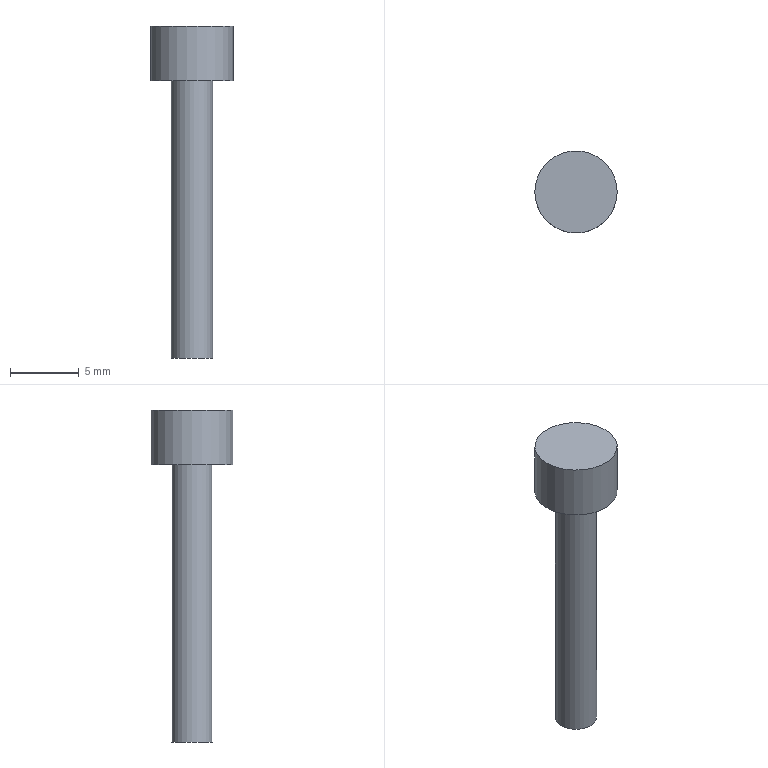Part | STEP file | 1 solid | 5 faces | box 6 x 6 x 24.2 mm | volume 255.883 mm3 | plane 3 | cylinder 2 | commonest cylinder face diameters 3 x1 6 x1
STEP:
#1=CARTESIAN_POINT('',(0.,0.,0.));
#2=DIRECTION('',(0.,0.,1.));
#3=DIRECTION('',(1.,0.,0.));
#4=AXIS2_PLACEMENT_3D('',#1,#2,#3);
#5=CARTESIAN_POINT('',(1542.983,484.48,23.419));
#6=VERTEX_POINT('',#5);
#7=CARTESIAN_POINT('',(1544.483,484.48,23.419));
#8=DIRECTION('',(0.,0.,1.));
#9=DIRECTION('',(-1.,0.,0.));
#10=AXIS2_PLACEMENT_3D('',#7,#8,#9);
#11=CIRCLE('',#10,1.5);
#12=CARTESIAN_POINT('',(1544.483,484.48,23.419));
#13=DIRECTION('',(0.,0.,-1.));
#14=DIRECTION('',(-1.,0.,0.));
#15=AXIS2_PLACEMENT_3D('',#12,#13,#14);
#16=PLANE('',#15);
#17=CARTESIAN_POINT('',(1.5,0.));
#18=CARTESIAN_POINT('',(1.5,-2.598));
#19=CARTESIAN_POINT('',(-0.75,-1.299));
#20=CARTESIAN_POINT('',(-3.,0.));
#21=CARTESIAN_POINT('',(-0.75,1.299));
#22=CARTESIAN_POINT('',(1.5,2.598));
#23=CARTESIAN_POINT('',(1.5,0.));
#24=(BOUNDED_CURVE()B_SPLINE_CURVE(2,(#17,#18,#19,#20,#21,#22,#23),.UNSPECIFIED.,.T.,.F.)B_SPLINE_CURVE_WITH_KNOTS((1,2,2,2,2,1),(-2.094,0.,2.094,4.189,6.283,8.378),.UNSPECIFIED.)CURVE()GEOMETRIC_REPRESENTATION_ITEM()RATIONAL_B_SPLINE_CURVE((1.,0.5,1.,0.5,1.,0.5,1.))REPRESENTATION_ITEM(''));
#25=(GEOMETRIC_REPRESENTATION_CONTEXT(2)PARAMETRIC_REPRESENTATION_CONTEXT()REPRESENTATION_CONTEXT('',''));
#26=DEFINITIONAL_REPRESENTATION('',(#24),#25);
#27=PCURVE('',#16,#26);
#28=CARTESIAN_POINT('',(1544.483,484.48,43.419));
#29=DIRECTION('',(0.,0.,-1.));
#30=DIRECTION('',(-1.,0.,0.));
#31=AXIS2_PLACEMENT_3D('',#28,#29,#30);
#32=CYLINDRICAL_SURFACE('',#31,1.5);
#33=CARTESIAN_POINT('',(6.283,20.));
#34=DIRECTION('',(-1.,0.));
#35=VECTOR('',#34,1.);
#36=LINE('',#33,#35);
#37=(GEOMETRIC_REPRESENTATION_CONTEXT(2)PARAMETRIC_REPRESENTATION_CONTEXT()REPRESENTATION_CONTEXT('',''));
#38=DEFINITIONAL_REPRESENTATION('',(#36),#37);
#39=PCURVE('',#32,#38);
#40=SURFACE_CURVE('',#11,(#27,#39),.PCURVE_S1.);
#41=EDGE_CURVE('',#6,#6,#40,.T.);
#42=ORIENTED_EDGE('',*,*,#41,.F.);
#43=EDGE_LOOP('',(#42));
#44=FACE_BOUND('',#43,.T.);
#45=ADVANCED_FACE('',(#44),#16,.T.);
#46=ORIENTED_EDGE('',*,*,#41,.T.);
#47=CARTESIAN_POINT('',(1542.983,484.48,43.619));
#48=VERTEX_POINT('',#47);
#49=CARTESIAN_POINT('',(1542.983,484.48,43.619));
#50=CARTESIAN_POINT('',(1542.983,484.48,23.419));
#51=B_SPLINE_CURVE_WITH_KNOTS('',1,(#49,#50),.UNSPECIFIED.,.F.,.F.,(2,2),(-0.2,20.),.PIECEWISE_BEZIER_KNOTS.);
#52=CARTESIAN_POINT('',(0.,0.));
#53=DIRECTION('',(0.,1.));
#54=VECTOR('',#53,1.);
#55=LINE('',#52,#54);
#56=(GEOMETRIC_REPRESENTATION_CONTEXT(2)PARAMETRIC_REPRESENTATION_CONTEXT()REPRESENTATION_CONTEXT('',''));
#57=DEFINITIONAL_REPRESENTATION('',(#55),#56);
#58=PCURVE('',#32,#57);
#59=CARTESIAN_POINT('',(6.283,0.));
#60=DIRECTION('',(0.,1.));
#61=VECTOR('',#60,1.);
#62=LINE('',#59,#61);
#63=(GEOMETRIC_REPRESENTATION_CONTEXT(2)PARAMETRIC_REPRESENTATION_CONTEXT()REPRESENTATION_CONTEXT('',''));
#64=DEFINITIONAL_REPRESENTATION('',(#62),#63);
#65=PCURVE('',#32,#64);
#66=SEAM_CURVE('',#51,(#58,#65),.PCURVE_S1.);
#67=EDGE_CURVE('',#48,#6,#66,.T.);
#68=ORIENTED_EDGE('',*,*,#67,.F.);
#69=CARTESIAN_POINT('',(1545.983,484.48,43.619));
#70=VERTEX_POINT('',#69);
#71=CARTESIAN_POINT('',(1544.483,484.48,43.619));
#72=DIRECTION('',(0.,0.,1.));
#73=DIRECTION('',(1.,0.,0.));
#74=AXIS2_PLACEMENT_3D('',#71,#72,#73);
#75=CIRCLE('',#74,1.5);
#76=CARTESIAN_POINT('',(3.142,-0.2));
#77=DIRECTION('',(-1.,0.));
#78=VECTOR('',#77,1.);
#79=LINE('',#76,#78);
#80=(GEOMETRIC_REPRESENTATION_CONTEXT(2)PARAMETRIC_REPRESENTATION_CONTEXT()REPRESENTATION_CONTEXT('',''));
#81=DEFINITIONAL_REPRESENTATION('',(#79),#80);
#82=PCURVE('',#32,#81);
#83=CARTESIAN_POINT('',(1544.483,484.48,43.619));
#84=DIRECTION('',(0.,0.,-1.));
#85=DIRECTION('',(-1.,0.,0.));
#86=AXIS2_PLACEMENT_3D('',#83,#84,#85);
#87=PLANE('',#86);
#88=CARTESIAN_POINT('',(-1.5,0.));
#89=CARTESIAN_POINT('',(-1.5,2.598));
#90=CARTESIAN_POINT('',(0.75,1.299));
#91=CARTESIAN_POINT('',(3.,0.));
#92=CARTESIAN_POINT('',(0.75,-1.299));
#93=CARTESIAN_POINT('',(-1.5,-2.598));
#94=CARTESIAN_POINT('',(-1.5,0.));
#95=(BOUNDED_CURVE()B_SPLINE_CURVE(2,(#88,#89,#90,#91,#92,#93,#94),.UNSPECIFIED.,.T.,.F.)B_SPLINE_CURVE_WITH_KNOTS((1,2,2,2,2,1),(-2.094,0.,2.094,4.189,6.283,8.378),.UNSPECIFIED.)CURVE()GEOMETRIC_REPRESENTATION_ITEM()RATIONAL_B_SPLINE_CURVE((1.,0.5,1.,0.5,1.,0.5,1.))REPRESENTATION_ITEM(''));
#96=(GEOMETRIC_REPRESENTATION_CONTEXT(2)PARAMETRIC_REPRESENTATION_CONTEXT()REPRESENTATION_CONTEXT('',''));
#97=DEFINITIONAL_REPRESENTATION('',(#95),#96);
#98=PCURVE('',#87,#97);
#99=SURFACE_CURVE('',#75,(#82,#98),.PCURVE_S1.);
#100=EDGE_CURVE('',#70,#48,#99,.T.);
#101=ORIENTED_EDGE('',*,*,#100,.F.);
#102=CARTESIAN_POINT('',(1544.483,484.48,43.619));
#103=DIRECTION('',(0.,0.,1.));
#104=DIRECTION('',(1.,0.,0.));
#105=AXIS2_PLACEMENT_3D('',#102,#103,#104);
#106=CIRCLE('',#105,1.5);
#107=CARTESIAN_POINT('',(9.425,-0.2));
#108=DIRECTION('',(-1.,0.));
#109=VECTOR('',#108,1.);
#110=LINE('',#107,#109);
#111=(GEOMETRIC_REPRESENTATION_CONTEXT(2)PARAMETRIC_REPRESENTATION_CONTEXT()REPRESENTATION_CONTEXT('',''));
#112=DEFINITIONAL_REPRESENTATION('',(#110),#111);
#113=PCURVE('',#32,#112);
#114=CARTESIAN_POINT('',(-1.5,0.));
#115=CARTESIAN_POINT('',(-1.5,2.598));
#116=CARTESIAN_POINT('',(0.75,1.299));
#117=CARTESIAN_POINT('',(3.,0.));
#118=CARTESIAN_POINT('',(0.75,-1.299));
#119=CARTESIAN_POINT('',(-1.5,-2.598));
#120=CARTESIAN_POINT('',(-1.5,0.));
#121=(BOUNDED_CURVE()B_SPLINE_CURVE(2,(#114,#115,#116,#117,#118,#119,#120),.UNSPECIFIED.,.T.,.F.)B_SPLINE_CURVE_WITH_KNOTS((1,2,2,2,2,1),(-2.094,0.,2.094,4.189,6.283,8.378),.UNSPECIFIED.)CURVE()GEOMETRIC_REPRESENTATION_ITEM()RATIONAL_B_SPLINE_CURVE((1.,0.5,1.,0.5,1.,0.5,1.))REPRESENTATION_ITEM(''));
#122=(GEOMETRIC_REPRESENTATION_CONTEXT(2)PARAMETRIC_REPRESENTATION_CONTEXT()REPRESENTATION_CONTEXT('',''));
#123=DEFINITIONAL_REPRESENTATION('',(#121),#122);
#124=PCURVE('',#87,#123);
#125=SURFACE_CURVE('',#106,(#113,#124),.PCURVE_S1.);
#126=EDGE_CURVE('',#48,#70,#125,.T.);
#127=ORIENTED_EDGE('',*,*,#126,.F.);
#128=ORIENTED_EDGE('',*,*,#67,.T.);
#129=EDGE_LOOP('',(#46,#68,#101,#127,#128));
#130=FACE_BOUND('',#129,.T.);
#131=ADVANCED_FACE('',(#130),#32,.T.);
#132=CARTESIAN_POINT('',(1541.483,484.48,47.619));
#133=VERTEX_POINT('',#132);
#134=CARTESIAN_POINT('',(1544.483,484.48,47.619));
#135=DIRECTION('',(0.,0.,-1.));
#136=DIRECTION('',(-1.,0.,0.));
#137=AXIS2_PLACEMENT_3D('',#134,#135,#136);
#138=CIRCLE('',#137,3.);
#139=CARTESIAN_POINT('',(1544.483,484.48,47.619));
#140=DIRECTION('',(0.,0.,1.));
#141=DIRECTION('',(1.,0.,0.));
#142=AXIS2_PLACEMENT_3D('',#139,#140,#141);
#143=PLANE('',#142);
#144=CARTESIAN_POINT('',(-3.,0.));
#145=CARTESIAN_POINT('',(-3.,5.196));
#146=CARTESIAN_POINT('',(1.5,2.598));
#147=CARTESIAN_POINT('',(6.,0.));
#148=CARTESIAN_POINT('',(1.5,-2.598));
#149=CARTESIAN_POINT('',(-3.,-5.196));
#150=CARTESIAN_POINT('',(-3.,0.));
#151=(BOUNDED_CURVE()B_SPLINE_CURVE(2,(#144,#145,#146,#147,#148,#149,#150),.UNSPECIFIED.,.T.,.F.)B_SPLINE_CURVE_WITH_KNOTS((1,2,2,2,2,1),(-2.094,0.,2.094,4.189,6.283,8.378),.UNSPECIFIED.)CURVE()GEOMETRIC_REPRESENTATION_ITEM()RATIONAL_B_SPLINE_CURVE((1.,0.5,1.,0.5,1.,0.5,1.))REPRESENTATION_ITEM(''));
#152=(GEOMETRIC_REPRESENTATION_CONTEXT(2)PARAMETRIC_REPRESENTATION_CONTEXT()REPRESENTATION_CONTEXT('',''));
#153=DEFINITIONAL_REPRESENTATION('',(#151),#152);
#154=PCURVE('',#143,#153);
#155=CARTESIAN_POINT('',(1544.483,484.48,43.619));
#156=DIRECTION('',(0.,0.,1.));
#157=DIRECTION('',(-1.,0.,0.));
#158=AXIS2_PLACEMENT_3D('',#155,#156,#157);
#159=CYLINDRICAL_SURFACE('',#158,3.);
#160=CARTESIAN_POINT('',(6.283,4.));
#161=DIRECTION('',(-1.,0.));
#162=VECTOR('',#161,1.);
#163=LINE('',#160,#162);
#164=(GEOMETRIC_REPRESENTATION_CONTEXT(2)PARAMETRIC_REPRESENTATION_CONTEXT()REPRESENTATION_CONTEXT('',''));
#165=DEFINITIONAL_REPRESENTATION('',(#163),#164);
#166=PCURVE('',#159,#165);
#167=SURFACE_CURVE('',#138,(#154,#166),.PCURVE_S1.);
#168=EDGE_CURVE('',#133,#133,#167,.T.);
#169=ORIENTED_EDGE('',*,*,#168,.F.);
#170=EDGE_LOOP('',(#169));
#171=FACE_BOUND('',#170,.T.);
#172=ADVANCED_FACE('',(#171),#143,.T.);
#173=ORIENTED_EDGE('',*,*,#100,.T.);
#174=ORIENTED_EDGE('',*,*,#126,.T.);
#175=EDGE_LOOP('',(#173,#174));
#176=FACE_BOUND('',#175,.T.);
#177=CARTESIAN_POINT('',(1547.483,484.48,43.619));
#178=VERTEX_POINT('',#177);
#179=CARTESIAN_POINT('',(1541.483,484.48,43.619));
#180=VERTEX_POINT('',#179);
#181=CARTESIAN_POINT('',(1544.483,484.48,43.619));
#182=DIRECTION('',(0.,0.,1.));
#183=DIRECTION('',(1.,0.,0.));
#184=AXIS2_PLACEMENT_3D('',#181,#182,#183);
#185=CIRCLE('',#184,3.);
#186=CARTESIAN_POINT('',(-3.,0.));
#187=CARTESIAN_POINT('',(-3.,5.196));
#188=CARTESIAN_POINT('',(1.5,2.598));
#189=CARTESIAN_POINT('',(6.,0.));
#190=CARTESIAN_POINT('',(1.5,-2.598));
#191=CARTESIAN_POINT('',(-3.,-5.196));
#192=CARTESIAN_POINT('',(-3.,0.));
#193=(BOUNDED_CURVE()B_SPLINE_CURVE(2,(#186,#187,#188,#189,#190,#191,#192),.UNSPECIFIED.,.T.,.F.)B_SPLINE_CURVE_WITH_KNOTS((1,2,2,2,2,1),(-2.094,0.,2.094,4.189,6.283,8.378),.UNSPECIFIED.)CURVE()GEOMETRIC_REPRESENTATION_ITEM()RATIONAL_B_SPLINE_CURVE((1.,0.5,1.,0.5,1.,0.5,1.))REPRESENTATION_ITEM(''));
#194=(GEOMETRIC_REPRESENTATION_CONTEXT(2)PARAMETRIC_REPRESENTATION_CONTEXT()REPRESENTATION_CONTEXT('',''));
#195=DEFINITIONAL_REPRESENTATION('',(#193),#194);
#196=PCURVE('',#87,#195);
#197=CARTESIAN_POINT('',(3.142,0.));
#198=DIRECTION('',(1.,0.));
#199=VECTOR('',#198,1.);
#200=LINE('',#197,#199);
#201=(GEOMETRIC_REPRESENTATION_CONTEXT(2)PARAMETRIC_REPRESENTATION_CONTEXT()REPRESENTATION_CONTEXT('',''));
#202=DEFINITIONAL_REPRESENTATION('',(#200),#201);
#203=PCURVE('',#159,#202);
#204=SURFACE_CURVE('',#185,(#196,#203),.PCURVE_S1.);
#205=EDGE_CURVE('',#178,#180,#204,.T.);
#206=ORIENTED_EDGE('',*,*,#205,.F.);
#207=CARTESIAN_POINT('',(1544.483,484.48,43.619));
#208=DIRECTION('',(0.,0.,1.));
#209=DIRECTION('',(1.,0.,0.));
#210=AXIS2_PLACEMENT_3D('',#207,#208,#209);
#211=CIRCLE('',#210,3.);
#212=CARTESIAN_POINT('',(-3.,0.));
#213=CARTESIAN_POINT('',(-3.,5.196));
#214=CARTESIAN_POINT('',(1.5,2.598));
#215=CARTESIAN_POINT('',(6.,0.));
#216=CARTESIAN_POINT('',(1.5,-2.598));
#217=CARTESIAN_POINT('',(-3.,-5.196));
#218=CARTESIAN_POINT('',(-3.,0.));
#219=(BOUNDED_CURVE()B_SPLINE_CURVE(2,(#212,#213,#214,#215,#216,#217,#218),.UNSPECIFIED.,.T.,.F.)B_SPLINE_CURVE_WITH_KNOTS((1,2,2,2,2,1),(-2.094,0.,2.094,4.189,6.283,8.378),.UNSPECIFIED.)CURVE()GEOMETRIC_REPRESENTATION_ITEM()RATIONAL_B_SPLINE_CURVE((1.,0.5,1.,0.5,1.,0.5,1.))REPRESENTATION_ITEM(''));
#220=(GEOMETRIC_REPRESENTATION_CONTEXT(2)PARAMETRIC_REPRESENTATION_CONTEXT()REPRESENTATION_CONTEXT('',''));
#221=DEFINITIONAL_REPRESENTATION('',(#219),#220);
#222=PCURVE('',#87,#221);
#223=CARTESIAN_POINT('',(-3.142,0.));
#224=DIRECTION('',(1.,0.));
#225=VECTOR('',#224,1.);
#226=LINE('',#223,#225);
#227=(GEOMETRIC_REPRESENTATION_CONTEXT(2)PARAMETRIC_REPRESENTATION_CONTEXT()REPRESENTATION_CONTEXT('',''));
#228=DEFINITIONAL_REPRESENTATION('',(#226),#227);
#229=PCURVE('',#159,#228);
#230=SURFACE_CURVE('',#211,(#222,#229),.PCURVE_S1.);
#231=EDGE_CURVE('',#180,#178,#230,.T.);
#232=ORIENTED_EDGE('',*,*,#231,.F.);
#233=EDGE_LOOP('',(#206,#232));
#234=FACE_BOUND('',#233,.T.);
#235=ADVANCED_FACE('',(#176,#234),#87,.T.);
#236=ORIENTED_EDGE('',*,*,#168,.T.);
#237=CARTESIAN_POINT('',(1541.483,484.48,43.619));
#238=CARTESIAN_POINT('',(1541.483,484.48,47.619));
#239=B_SPLINE_CURVE_WITH_KNOTS('',1,(#237,#238),.UNSPECIFIED.,.F.,.F.,(2,2),(0.,4.),.PIECEWISE_BEZIER_KNOTS.);
#240=CARTESIAN_POINT('',(0.,0.));
#241=DIRECTION('',(0.,1.));
#242=VECTOR('',#241,1.);
#243=LINE('',#240,#242);
#244=(GEOMETRIC_REPRESENTATION_CONTEXT(2)PARAMETRIC_REPRESENTATION_CONTEXT()REPRESENTATION_CONTEXT('',''));
#245=DEFINITIONAL_REPRESENTATION('',(#243),#244);
#246=PCURVE('',#159,#245);
#247=CARTESIAN_POINT('',(6.283,0.));
#248=DIRECTION('',(0.,1.));
#249=VECTOR('',#248,1.);
#250=LINE('',#247,#249);
#251=(GEOMETRIC_REPRESENTATION_CONTEXT(2)PARAMETRIC_REPRESENTATION_CONTEXT()REPRESENTATION_CONTEXT('',''));
#252=DEFINITIONAL_REPRESENTATION('',(#250),#251);
#253=PCURVE('',#159,#252);
#254=SEAM_CURVE('',#239,(#246,#253),.PCURVE_S1.);
#255=EDGE_CURVE('',#180,#133,#254,.T.);
#256=ORIENTED_EDGE('',*,*,#255,.F.);
#257=ORIENTED_EDGE('',*,*,#231,.T.);
#258=ORIENTED_EDGE('',*,*,#205,.T.);
#259=ORIENTED_EDGE('',*,*,#255,.T.);
#260=EDGE_LOOP('',(#236,#256,#257,#258,#259));
#261=FACE_BOUND('',#260,.T.);
#262=ADVANCED_FACE('',(#261),#159,.T.);
#263=CLOSED_SHELL('',(#45,#131,#172,#235,#262));
#264=MANIFOLD_SOLID_BREP('',#263);
#265=(LENGTH_UNIT()NAMED_UNIT(*)SI_UNIT(.MILLI.,.METRE.));
#266=UNCERTAINTY_MEASURE_WITH_UNIT(LENGTH_MEASURE(0.000005),#265,'','');
#267=(NAMED_UNIT(*)PLANE_ANGLE_UNIT()SI_UNIT($,.RADIAN.));
#268=(NAMED_UNIT(*)SI_UNIT($,.STERADIAN.)SOLID_ANGLE_UNIT());
#269=(GEOMETRIC_REPRESENTATION_CONTEXT(3)GLOBAL_UNCERTAINTY_ASSIGNED_CONTEXT((#266))GLOBAL_UNIT_ASSIGNED_CONTEXT((#265,#267,#268))REPRESENTATION_CONTEXT('',''));
#270=ADVANCED_BREP_SHAPE_REPRESENTATION('',(#4,#264),#269);